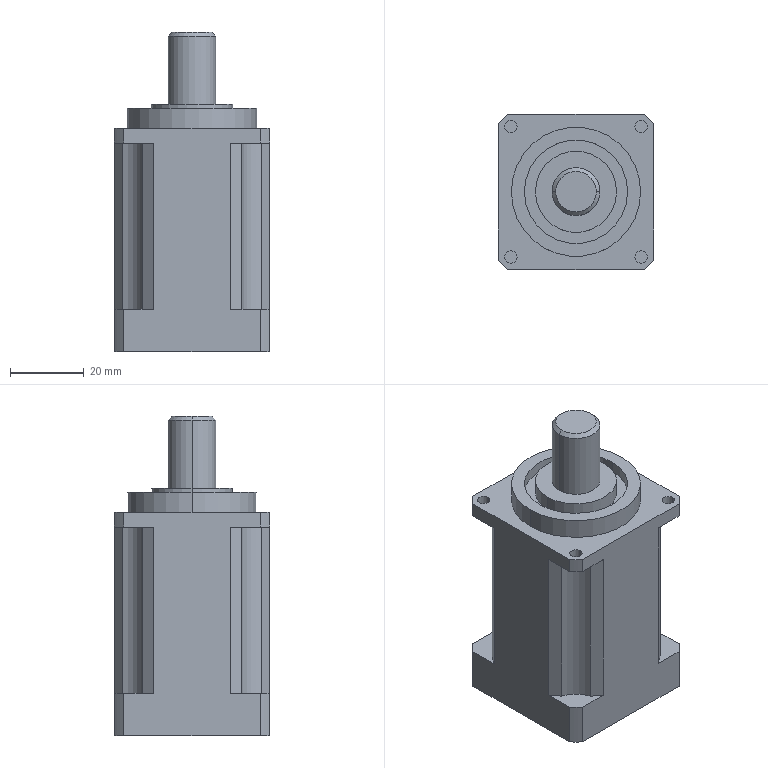Part | SolidWorks | features Boss 5, Cut 4, Chamfer 2, Extrusion 1 | 1 solid | 56 faces | box 42 x 42 x 86.5 mm | volume 103966 mm3 | cylinder 28 | plane 26 | cone 2 | commonest cylinder face diameters 3.4 x8 56 x8 16 x4 13 x2 22 x2 28 x2